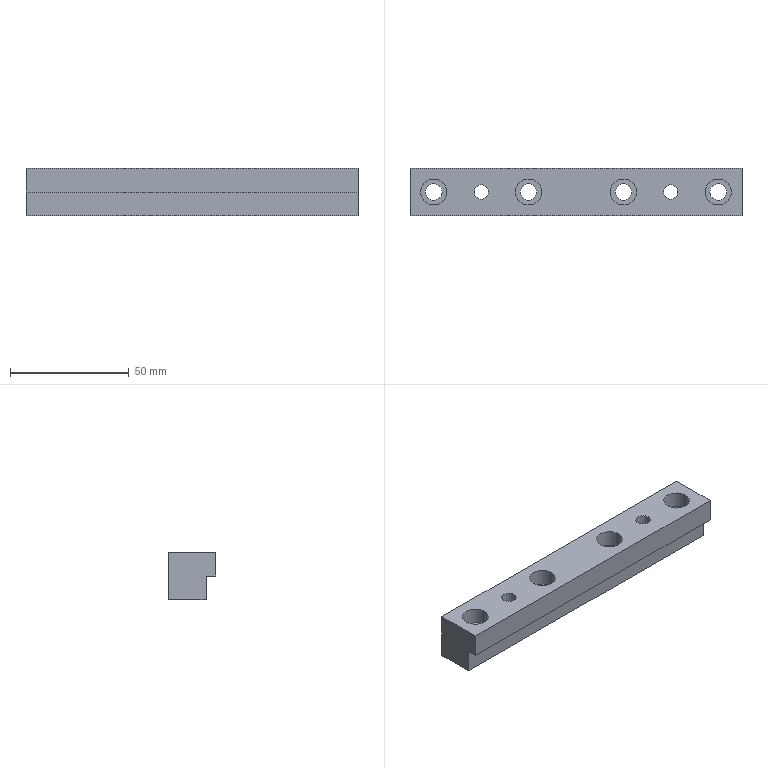Part | STEP file | 200 mesh_id1922 | 1 solid | 22 faces | box 140 x 20 x 20 mm | volume 44533 mm3 | plane 12 | cylinder 10 | commonest cylinder face diameters 7 x4 11 x4 6.01 x2
STEP:
#1=CARTESIAN_POINT('',(-16699.686,-3880.269,22.));
#2=VERTEX_POINT('',#1);
#3=CARTESIAN_POINT('',(-16839.686,-3880.269,22.));
#4=VERTEX_POINT('',#3);
#5=CARTESIAN_POINT('',(-16903.186,-3880.269,22.));
#6=DIRECTION('',(-1.,0.,0.));
#7=VECTOR('',#6,1.);
#8=LINE('',#5,#7);
#9=EDGE_CURVE('',#2,#4,#8,.T.);
#10=ORIENTED_EDGE('',*,*,#9,.F.);
#11=CARTESIAN_POINT('',(-16699.686,-3880.269,32.));
#12=VERTEX_POINT('',#11);
#13=CARTESIAN_POINT('',(-16699.686,-3880.269,12.));
#14=DIRECTION('',(0.,0.,-1.));
#15=VECTOR('',#14,1.);
#16=LINE('',#13,#15);
#17=EDGE_CURVE('',#12,#2,#16,.T.);
#18=ORIENTED_EDGE('',*,*,#17,.F.);
#19=CARTESIAN_POINT('',(-16839.686,-3880.269,32.));
#20=VERTEX_POINT('',#19);
#21=CARTESIAN_POINT('',(-16841.186,-3880.269,32.));
#22=DIRECTION('',(-1.,0.,0.));
#23=VECTOR('',#22,1.);
#24=LINE('',#21,#23);
#25=EDGE_CURVE('',#12,#20,#24,.T.);
#26=ORIENTED_EDGE('',*,*,#25,.T.);
#27=CARTESIAN_POINT('',(-16839.686,-3880.269,12.));
#28=DIRECTION('',(0.,0.,-1.));
#29=VECTOR('',#28,1.);
#30=LINE('',#27,#29);
#31=EDGE_CURVE('',#20,#4,#30,.T.);
#32=ORIENTED_EDGE('',*,*,#31,.T.);
#33=EDGE_LOOP('',(#10,#18,#26,#32));
#34=FACE_OUTER_BOUND('',#33,.T.);
#35=CARTESIAN_POINT('',(-16841.186,-3880.269,12.));
#36=DIRECTION('',(0.,1.,0.));
#37=DIRECTION('',(0.,0.,-1.));
#38=AXIS2_PLACEMENT_3D('',#35,#36,#37);
#39=PLANE('',#38);
#40=ADVANCED_FACE('',(#34),#39,.F.);
#41=CARTESIAN_POINT('',(-16699.686,-3876.219,12.));
#42=VERTEX_POINT('',#41);
#43=CARTESIAN_POINT('',(-16699.686,-3876.219,22.));
#44=VERTEX_POINT('',#43);
#45=CARTESIAN_POINT('',(-16699.686,-3876.219,22.));
#46=DIRECTION('',(0.,0.,1.));
#47=VECTOR('',#46,1.);
#48=LINE('',#45,#47);
#49=EDGE_CURVE('',#42,#44,#48,.T.);
#50=ORIENTED_EDGE('',*,*,#49,.F.);
#51=CARTESIAN_POINT('',(-16699.686,-3860.269,12.));
#52=VERTEX_POINT('',#51);
#53=CARTESIAN_POINT('',(-16699.686,-3870.269,12.));
#54=DIRECTION('',(0.,-1.,0.));
#55=VECTOR('',#54,1.);
#56=LINE('',#53,#55);
#57=EDGE_CURVE('',#52,#42,#56,.T.);
#58=ORIENTED_EDGE('',*,*,#57,.F.);
#59=CARTESIAN_POINT('',(-16699.686,-3860.269,32.));
#60=VERTEX_POINT('',#59);
#61=CARTESIAN_POINT('',(-16699.686,-3860.269,12.));
#62=DIRECTION('',(0.,0.,-1.));
#63=VECTOR('',#62,1.);
#64=LINE('',#61,#63);
#65=EDGE_CURVE('',#60,#52,#64,.T.);
#66=ORIENTED_EDGE('',*,*,#65,.F.);
#67=CARTESIAN_POINT('',(-16699.686,-3870.269,32.));
#68=DIRECTION('',(0.,-1.,0.));
#69=VECTOR('',#68,1.);
#70=LINE('',#67,#69);
#71=EDGE_CURVE('',#60,#12,#70,.T.);
#72=ORIENTED_EDGE('',*,*,#71,.T.);
#73=ORIENTED_EDGE('',*,*,#17,.T.);
#74=CARTESIAN_POINT('',(-16699.686,-3880.269,22.));
#75=DIRECTION('',(0.,-1.,0.));
#76=VECTOR('',#75,1.);
#77=LINE('',#74,#76);
#78=EDGE_CURVE('',#44,#2,#77,.T.);
#79=ORIENTED_EDGE('',*,*,#78,.F.);
#80=EDGE_LOOP('',(#50,#58,#66,#72,#73,#79));
#81=FACE_OUTER_BOUND('',#80,.T.);
#82=CARTESIAN_POINT('',(-16699.686,-3880.269,12.));
#83=DIRECTION('',(-1.,0.,0.));
#84=DIRECTION('',(0.,1.,0.));
#85=AXIS2_PLACEMENT_3D('',#82,#83,#84);
#86=PLANE('',#85);
#87=ADVANCED_FACE('',(#81),#86,.F.);
#88=CARTESIAN_POINT('',(-16826.186,-3870.269,12.));
#89=VERTEX_POINT('',#88);
#90=CARTESIAN_POINT('',(-16829.686,-3870.269,12.));
#91=DIRECTION('',(0.,0.,1.));
#92=DIRECTION('',(1.,0.,0.));
#93=AXIS2_PLACEMENT_3D('',#90,#91,#92);
#94=CIRCLE('',#93,3.5);
#95=EDGE_CURVE('',#89,#89,#94,.T.);
#96=ORIENTED_EDGE('',*,*,#95,.T.);
#97=EDGE_LOOP('',(#96));
#98=FACE_BOUND('',#97,.T.);
#99=CARTESIAN_POINT('',(-16806.681,-3870.269,12.));
#100=VERTEX_POINT('',#99);
#101=CARTESIAN_POINT('',(-16809.686,-3870.269,12.));
#102=DIRECTION('',(0.,0.,1.));
#103=DIRECTION('',(1.,0.,0.));
#104=AXIS2_PLACEMENT_3D('',#101,#102,#103);
#105=CIRCLE('',#104,3.005);
#106=EDGE_CURVE('',#100,#100,#105,.T.);
#107=ORIENTED_EDGE('',*,*,#106,.T.);
#108=EDGE_LOOP('',(#107));
#109=FACE_BOUND('',#108,.T.);
#110=CARTESIAN_POINT('',(-16786.186,-3870.269,12.));
#111=VERTEX_POINT('',#110);
#112=CARTESIAN_POINT('',(-16789.686,-3870.269,12.));
#113=DIRECTION('',(0.,0.,1.));
#114=DIRECTION('',(1.,0.,0.));
#115=AXIS2_PLACEMENT_3D('',#112,#113,#114);
#116=CIRCLE('',#115,3.5);
#117=EDGE_CURVE('',#111,#111,#116,.T.);
#118=ORIENTED_EDGE('',*,*,#117,.T.);
#119=EDGE_LOOP('',(#118));
#120=FACE_BOUND('',#119,.T.);
#121=CARTESIAN_POINT('',(-16726.681,-3870.269,12.));
#122=VERTEX_POINT('',#121);
#123=CARTESIAN_POINT('',(-16729.686,-3870.269,12.));
#124=DIRECTION('',(0.,0.,1.));
#125=DIRECTION('',(1.,0.,0.));
#126=AXIS2_PLACEMENT_3D('',#123,#124,#125);
#127=CIRCLE('',#126,3.005);
#128=EDGE_CURVE('',#122,#122,#127,.T.);
#129=ORIENTED_EDGE('',*,*,#128,.T.);
#130=EDGE_LOOP('',(#129));
#131=FACE_BOUND('',#130,.T.);
#132=CARTESIAN_POINT('',(-16746.186,-3870.269,12.));
#133=VERTEX_POINT('',#132);
#134=CARTESIAN_POINT('',(-16749.686,-3870.269,12.));
#135=DIRECTION('',(0.,0.,1.));
#136=DIRECTION('',(1.,0.,0.));
#137=AXIS2_PLACEMENT_3D('',#134,#135,#136);
#138=CIRCLE('',#137,3.5);
#139=EDGE_CURVE('',#133,#133,#138,.T.);
#140=ORIENTED_EDGE('',*,*,#139,.T.);
#141=EDGE_LOOP('',(#140));
#142=FACE_BOUND('',#141,.T.);
#143=CARTESIAN_POINT('',(-16706.186,-3870.269,12.));
#144=VERTEX_POINT('',#143);
#145=CARTESIAN_POINT('',(-16709.686,-3870.269,12.));
#146=DIRECTION('',(0.,0.,1.));
#147=DIRECTION('',(1.,0.,0.));
#148=AXIS2_PLACEMENT_3D('',#145,#146,#147);
#149=CIRCLE('',#148,3.5);
#150=EDGE_CURVE('',#144,#144,#149,.T.);
#151=ORIENTED_EDGE('',*,*,#150,.T.);
#152=EDGE_LOOP('',(#151));
#153=FACE_BOUND('',#152,.T.);
#154=CARTESIAN_POINT('',(-16839.686,-3876.219,12.));
#155=VERTEX_POINT('',#154);
#156=CARTESIAN_POINT('',(-16903.186,-3876.219,12.));
#157=DIRECTION('',(1.,0.,0.));
#158=VECTOR('',#157,1.);
#159=LINE('',#156,#158);
#160=EDGE_CURVE('',#155,#42,#159,.T.);
#161=ORIENTED_EDGE('',*,*,#160,.F.);
#162=CARTESIAN_POINT('',(-16839.686,-3860.269,12.));
#163=VERTEX_POINT('',#162);
#164=CARTESIAN_POINT('',(-16839.686,-3870.269,12.));
#165=DIRECTION('',(0.,1.,0.));
#166=VECTOR('',#165,1.);
#167=LINE('',#164,#166);
#168=EDGE_CURVE('',#155,#163,#167,.T.);
#169=ORIENTED_EDGE('',*,*,#168,.T.);
#170=CARTESIAN_POINT('',(-16703.186,-3860.269,12.));
#171=DIRECTION('',(1.,0.,0.));
#172=VECTOR('',#171,1.);
#173=LINE('',#170,#172);
#174=EDGE_CURVE('',#163,#52,#173,.T.);
#175=ORIENTED_EDGE('',*,*,#174,.T.);
#176=ORIENTED_EDGE('',*,*,#57,.T.);
#177=EDGE_LOOP('',(#161,#169,#175,#176));
#178=FACE_BOUND('',#177,.T.);
#179=CARTESIAN_POINT('',(-16709.686,-3870.269,12.));
#180=DIRECTION('',(0.,0.,1.));
#181=DIRECTION('',(1.,0.,0.));
#182=AXIS2_PLACEMENT_3D('',#179,#180,#181);
#183=PLANE('',#182);
#184=ADVANCED_FACE('',(#98,#109,#120,#131,#142,#153,#178),#183,.F.);
#185=CARTESIAN_POINT('',(-16839.686,-3876.219,22.));
#186=VERTEX_POINT('',#185);
#187=CARTESIAN_POINT('',(-16839.686,-3860.269,22.));
#188=DIRECTION('',(0.,-1.,0.));
#189=VECTOR('',#188,1.);
#190=LINE('',#187,#189);
#191=EDGE_CURVE('',#186,#4,#190,.T.);
#192=ORIENTED_EDGE('',*,*,#191,.T.);
#193=ORIENTED_EDGE('',*,*,#31,.F.);
#194=CARTESIAN_POINT('',(-16839.686,-3860.269,32.));
#195=VERTEX_POINT('',#194);
#196=CARTESIAN_POINT('',(-16839.686,-3870.269,32.));
#197=DIRECTION('',(0.,1.,0.));
#198=VECTOR('',#197,1.);
#199=LINE('',#196,#198);
#200=EDGE_CURVE('',#20,#195,#199,.T.);
#201=ORIENTED_EDGE('',*,*,#200,.T.);
#202=CARTESIAN_POINT('',(-16839.686,-3860.269,12.));
#203=DIRECTION('',(0.,0.,-1.));
#204=VECTOR('',#203,1.);
#205=LINE('',#202,#204);
#206=EDGE_CURVE('',#195,#163,#205,.T.);
#207=ORIENTED_EDGE('',*,*,#206,.T.);
#208=ORIENTED_EDGE('',*,*,#168,.F.);
#209=CARTESIAN_POINT('',(-16839.686,-3876.219,12.));
#210=DIRECTION('',(0.,0.,1.));
#211=VECTOR('',#210,1.);
#212=LINE('',#209,#211);
#213=EDGE_CURVE('',#155,#186,#212,.T.);
#214=ORIENTED_EDGE('',*,*,#213,.T.);
#215=EDGE_LOOP('',(#192,#193,#201,#207,#208,#214));
#216=FACE_OUTER_BOUND('',#215,.T.);
#217=CARTESIAN_POINT('',(-16839.686,-3860.269,12.));
#218=DIRECTION('',(1.,0.,0.));
#219=DIRECTION('',(0.,0.,-1.));
#220=AXIS2_PLACEMENT_3D('',#217,#218,#219);
#221=PLANE('',#220);
#222=ADVANCED_FACE('',(#216),#221,.F.);
#223=ORIENTED_EDGE('',*,*,#106,.F.);
#224=EDGE_LOOP('',(#223));
#225=FACE_BOUND('',#224,.T.);
#226=CARTESIAN_POINT('',(-16806.681,-3870.269,32.));
#227=VERTEX_POINT('',#226);
#228=CARTESIAN_POINT('',(-16809.686,-3870.269,32.));
#229=DIRECTION('',(0.,0.,1.));
#230=DIRECTION('',(1.,0.,0.));
#231=AXIS2_PLACEMENT_3D('',#228,#229,#230);
#232=CIRCLE('',#231,3.005);
#233=EDGE_CURVE('',#227,#227,#232,.T.);
#234=ORIENTED_EDGE('',*,*,#233,.T.);
#235=EDGE_LOOP('',(#234));
#236=FACE_BOUND('',#235,.T.);
#237=CARTESIAN_POINT('',(-16809.686,-3870.269,12.));
#238=DIRECTION('',(0.,0.,1.));
#239=DIRECTION('',(1.,0.,0.));
#240=AXIS2_PLACEMENT_3D('',#237,#238,#239);
#241=CYLINDRICAL_SURFACE('',#240,3.005);
#242=ADVANCED_FACE('',(#225,#236),#241,.F.);
#243=CARTESIAN_POINT('',(-16793.186,-3870.269,25.));
#244=VERTEX_POINT('',#243);
#245=CARTESIAN_POINT('',(-16789.686,-3870.269,25.));
#246=DIRECTION('',(0.,0.,1.));
#247=DIRECTION('',(-1.,0.,0.));
#248=AXIS2_PLACEMENT_3D('',#245,#246,#247);
#249=CIRCLE('',#248,3.5);
#250=EDGE_CURVE('',#244,#244,#249,.T.);
#251=ORIENTED_EDGE('',*,*,#250,.T.);
#252=EDGE_LOOP('',(#251));
#253=FACE_BOUND('',#252,.T.);
#254=ORIENTED_EDGE('',*,*,#117,.F.);
#255=EDGE_LOOP('',(#254));
#256=FACE_BOUND('',#255,.T.);
#257=CARTESIAN_POINT('',(-16789.686,-3870.269,12.));
#258=DIRECTION('',(0.,0.,1.));
#259=DIRECTION('',(1.,0.,0.));
#260=AXIS2_PLACEMENT_3D('',#257,#258,#259);
#261=CYLINDRICAL_SURFACE('',#260,3.5);
#262=ADVANCED_FACE('',(#253,#256),#261,.F.);
#263=ORIENTED_EDGE('',*,*,#128,.F.);
#264=EDGE_LOOP('',(#263));
#265=FACE_BOUND('',#264,.T.);
#266=CARTESIAN_POINT('',(-16726.681,-3870.269,32.));
#267=VERTEX_POINT('',#266);
#268=CARTESIAN_POINT('',(-16729.686,-3870.269,32.));
#269=DIRECTION('',(0.,0.,1.));
#270=DIRECTION('',(1.,0.,0.));
#271=AXIS2_PLACEMENT_3D('',#268,#269,#270);
#272=CIRCLE('',#271,3.005);
#273=EDGE_CURVE('',#267,#267,#272,.T.);
#274=ORIENTED_EDGE('',*,*,#273,.T.);
#275=EDGE_LOOP('',(#274));
#276=FACE_BOUND('',#275,.T.);
#277=CARTESIAN_POINT('',(-16729.686,-3870.269,12.));
#278=DIRECTION('',(0.,0.,1.));
#279=DIRECTION('',(1.,0.,0.));
#280=AXIS2_PLACEMENT_3D('',#277,#278,#279);
#281=CYLINDRICAL_SURFACE('',#280,3.005);
#282=ADVANCED_FACE('',(#265,#276),#281,.F.);
#283=CARTESIAN_POINT('',(-16753.186,-3870.269,25.));
#284=VERTEX_POINT('',#283);
#285=CARTESIAN_POINT('',(-16749.686,-3870.269,25.));
#286=DIRECTION('',(0.,0.,1.));
#287=DIRECTION('',(-1.,0.,0.));
#288=AXIS2_PLACEMENT_3D('',#285,#286,#287);
#289=CIRCLE('',#288,3.5);
#290=EDGE_CURVE('',#284,#284,#289,.T.);
#291=ORIENTED_EDGE('',*,*,#290,.T.);
#292=EDGE_LOOP('',(#291));
#293=FACE_BOUND('',#292,.T.);
#294=ORIENTED_EDGE('',*,*,#139,.F.);
#295=EDGE_LOOP('',(#294));
#296=FACE_BOUND('',#295,.T.);
#297=CARTESIAN_POINT('',(-16749.686,-3870.269,12.));
#298=DIRECTION('',(0.,0.,1.));
#299=DIRECTION('',(1.,0.,0.));
#300=AXIS2_PLACEMENT_3D('',#297,#298,#299);
#301=CYLINDRICAL_SURFACE('',#300,3.5);
#302=ADVANCED_FACE('',(#293,#296),#301,.F.);
#303=CARTESIAN_POINT('',(-16713.186,-3870.269,25.));
#304=VERTEX_POINT('',#303);
#305=CARTESIAN_POINT('',(-16709.686,-3870.269,25.));
#306=DIRECTION('',(0.,0.,1.));
#307=DIRECTION('',(-1.,0.,0.));
#308=AXIS2_PLACEMENT_3D('',#305,#306,#307);
#309=CIRCLE('',#308,3.5);
#310=EDGE_CURVE('',#304,#304,#309,.T.);
#311=ORIENTED_EDGE('',*,*,#310,.T.);
#312=EDGE_LOOP('',(#311));
#313=FACE_BOUND('',#312,.T.);
#314=ORIENTED_EDGE('',*,*,#150,.F.);
#315=EDGE_LOOP('',(#314));
#316=FACE_BOUND('',#315,.T.);
#317=CARTESIAN_POINT('',(-16709.686,-3870.269,12.));
#318=DIRECTION('',(0.,0.,1.));
#319=DIRECTION('',(1.,0.,0.));
#320=AXIS2_PLACEMENT_3D('',#317,#318,#319);
#321=CYLINDRICAL_SURFACE('',#320,3.5);
#322=ADVANCED_FACE('',(#313,#316),#321,.F.);
#323=CARTESIAN_POINT('',(-16703.186,-3860.269,32.));
#324=DIRECTION('',(1.,0.,0.));
#325=VECTOR('',#324,1.);
#326=LINE('',#323,#325);
#327=EDGE_CURVE('',#195,#60,#326,.T.);
#328=ORIENTED_EDGE('',*,*,#327,.T.);
#329=ORIENTED_EDGE('',*,*,#65,.T.);
#330=ORIENTED_EDGE('',*,*,#174,.F.);
#331=ORIENTED_EDGE('',*,*,#206,.F.);
#332=EDGE_LOOP('',(#328,#329,#330,#331));
#333=FACE_OUTER_BOUND('',#332,.T.);
#334=CARTESIAN_POINT('',(-16703.186,-3860.269,12.));
#335=DIRECTION('',(0.,-1.,0.));
#336=DIRECTION('',(-1.,0.,0.));
#337=AXIS2_PLACEMENT_3D('',#334,#335,#336);
#338=PLANE('',#337);
#339=ADVANCED_FACE('',(#333),#338,.F.);
#340=CARTESIAN_POINT('',(-16833.186,-3870.269,25.));
#341=VERTEX_POINT('',#340);
#342=CARTESIAN_POINT('',(-16829.686,-3870.269,25.));
#343=DIRECTION('',(0.,0.,1.));
#344=DIRECTION('',(-1.,0.,0.));
#345=AXIS2_PLACEMENT_3D('',#342,#343,#344);
#346=CIRCLE('',#345,3.5);
#347=EDGE_CURVE('',#341,#341,#346,.T.);
#348=ORIENTED_EDGE('',*,*,#347,.T.);
#349=EDGE_LOOP('',(#348));
#350=FACE_BOUND('',#349,.T.);
#351=ORIENTED_EDGE('',*,*,#95,.F.);
#352=EDGE_LOOP('',(#351));
#353=FACE_BOUND('',#352,.T.);
#354=CARTESIAN_POINT('',(-16829.686,-3870.269,12.));
#355=DIRECTION('',(0.,0.,1.));
#356=DIRECTION('',(1.,0.,0.));
#357=AXIS2_PLACEMENT_3D('',#354,#355,#356);
#358=CYLINDRICAL_SURFACE('',#357,3.5);
#359=ADVANCED_FACE('',(#350,#353),#358,.F.);
#360=CARTESIAN_POINT('',(-16704.186,-3870.269,32.));
#361=VERTEX_POINT('',#360);
#362=CARTESIAN_POINT('',(-16709.686,-3870.269,32.));
#363=DIRECTION('',(0.,0.,-1.));
#364=DIRECTION('',(1.,0.,0.));
#365=AXIS2_PLACEMENT_3D('',#362,#363,#364);
#366=CIRCLE('',#365,5.5);
#367=EDGE_CURVE('',#361,#361,#366,.T.);
#368=ORIENTED_EDGE('',*,*,#367,.T.);
#369=EDGE_LOOP('',(#368));
#370=FACE_BOUND('',#369,.T.);
#371=CARTESIAN_POINT('',(-16744.186,-3870.269,32.));
#372=VERTEX_POINT('',#371);
#373=CARTESIAN_POINT('',(-16749.686,-3870.269,32.));
#374=DIRECTION('',(0.,0.,-1.));
#375=DIRECTION('',(1.,0.,0.));
#376=AXIS2_PLACEMENT_3D('',#373,#374,#375);
#377=CIRCLE('',#376,5.5);
#378=EDGE_CURVE('',#372,#372,#377,.T.);
#379=ORIENTED_EDGE('',*,*,#378,.T.);
#380=EDGE_LOOP('',(#379));
#381=FACE_BOUND('',#380,.T.);
#382=CARTESIAN_POINT('',(-16784.186,-3870.269,32.));
#383=VERTEX_POINT('',#382);
#384=CARTESIAN_POINT('',(-16789.686,-3870.269,32.));
#385=DIRECTION('',(0.,0.,-1.));
#386=DIRECTION('',(1.,0.,0.));
#387=AXIS2_PLACEMENT_3D('',#384,#385,#386);
#388=CIRCLE('',#387,5.5);
#389=EDGE_CURVE('',#383,#383,#388,.T.);
#390=ORIENTED_EDGE('',*,*,#389,.T.);
#391=EDGE_LOOP('',(#390));
#392=FACE_BOUND('',#391,.T.);
#393=CARTESIAN_POINT('',(-16824.186,-3870.269,32.));
#394=VERTEX_POINT('',#393);
#395=CARTESIAN_POINT('',(-16829.686,-3870.269,32.));
#396=DIRECTION('',(0.,0.,-1.));
#397=DIRECTION('',(1.,0.,0.));
#398=AXIS2_PLACEMENT_3D('',#395,#396,#397);
#399=CIRCLE('',#398,5.5);
#400=EDGE_CURVE('',#394,#394,#399,.T.);
#401=ORIENTED_EDGE('',*,*,#400,.T.);
#402=EDGE_LOOP('',(#401));
#403=FACE_BOUND('',#402,.T.);
#404=ORIENTED_EDGE('',*,*,#200,.F.);
#405=ORIENTED_EDGE('',*,*,#25,.F.);
#406=ORIENTED_EDGE('',*,*,#71,.F.);
#407=ORIENTED_EDGE('',*,*,#327,.F.);
#408=EDGE_LOOP('',(#404,#405,#406,#407));
#409=FACE_BOUND('',#408,.T.);
#410=ORIENTED_EDGE('',*,*,#273,.F.);
#411=EDGE_LOOP('',(#410));
#412=FACE_BOUND('',#411,.T.);
#413=ORIENTED_EDGE('',*,*,#233,.F.);
#414=EDGE_LOOP('',(#413));
#415=FACE_BOUND('',#414,.T.);
#416=CARTESIAN_POINT('',(-16709.686,-3870.269,32.));
#417=DIRECTION('',(0.,0.,1.));
#418=DIRECTION('',(1.,0.,0.));
#419=AXIS2_PLACEMENT_3D('',#416,#417,#418);
#420=PLANE('',#419);
#421=ADVANCED_FACE('',(#370,#381,#392,#403,#409,#412,#415),#420,.T.);
#422=ORIENTED_EDGE('',*,*,#213,.F.);
#423=ORIENTED_EDGE('',*,*,#160,.T.);
#424=ORIENTED_EDGE('',*,*,#49,.T.);
#425=CARTESIAN_POINT('',(-16903.186,-3876.219,22.));
#426=DIRECTION('',(-1.,0.,0.));
#427=VECTOR('',#426,1.);
#428=LINE('',#425,#427);
#429=EDGE_CURVE('',#44,#186,#428,.T.);
#430=ORIENTED_EDGE('',*,*,#429,.T.);
#431=EDGE_LOOP('',(#422,#423,#424,#430));
#432=FACE_OUTER_BOUND('',#431,.T.);
#433=CARTESIAN_POINT('',(-16903.186,-3876.219,22.));
#434=DIRECTION('',(0.,1.,0.));
#435=DIRECTION('',(1.,0.,0.));
#436=AXIS2_PLACEMENT_3D('',#433,#434,#435);
#437=PLANE('',#436);
#438=ADVANCED_FACE('',(#432),#437,.F.);
#439=ORIENTED_EDGE('',*,*,#191,.F.);
#440=ORIENTED_EDGE('',*,*,#429,.F.);
#441=ORIENTED_EDGE('',*,*,#78,.T.);
#442=ORIENTED_EDGE('',*,*,#9,.T.);
#443=EDGE_LOOP('',(#439,#440,#441,#442));
#444=FACE_OUTER_BOUND('',#443,.T.);
#445=CARTESIAN_POINT('',(-16903.186,-3880.269,22.));
#446=DIRECTION('',(0.,0.,1.));
#447=DIRECTION('',(0.,-1.,0.));
#448=AXIS2_PLACEMENT_3D('',#445,#446,#447);
#449=PLANE('',#448);
#450=ADVANCED_FACE('',(#444),#449,.F.);
#451=CARTESIAN_POINT('',(-16835.186,-3870.269,25.));
#452=VERTEX_POINT('',#451);
#453=CARTESIAN_POINT('',(-16829.686,-3870.269,25.));
#454=DIRECTION('',(0.,0.,-1.));
#455=DIRECTION('',(-1.,0.,0.));
#456=AXIS2_PLACEMENT_3D('',#453,#454,#455);
#457=CIRCLE('',#456,5.5);
#458=EDGE_CURVE('',#452,#452,#457,.T.);
#459=ORIENTED_EDGE('',*,*,#458,.F.);
#460=EDGE_LOOP('',(#459));
#461=FACE_BOUND('',#460,.T.);
#462=ORIENTED_EDGE('',*,*,#347,.F.);
#463=EDGE_LOOP('',(#462));
#464=FACE_BOUND('',#463,.T.);
#465=CARTESIAN_POINT('',(-16829.686,-3870.269,25.));
#466=DIRECTION('',(0.,0.,-1.));
#467=DIRECTION('',(-1.,0.,0.));
#468=AXIS2_PLACEMENT_3D('',#465,#466,#467);
#469=PLANE('',#468);
#470=ADVANCED_FACE('',(#461,#464),#469,.F.);
#471=ORIENTED_EDGE('',*,*,#458,.T.);
#472=EDGE_LOOP('',(#471));
#473=FACE_BOUND('',#472,.T.);
#474=ORIENTED_EDGE('',*,*,#400,.F.);
#475=EDGE_LOOP('',(#474));
#476=FACE_BOUND('',#475,.T.);
#477=CARTESIAN_POINT('',(-16829.686,-3870.269,32.));
#478=DIRECTION('',(0.,0.,-1.));
#479=DIRECTION('',(1.,0.,0.));
#480=AXIS2_PLACEMENT_3D('',#477,#478,#479);
#481=CYLINDRICAL_SURFACE('',#480,5.5);
#482=ADVANCED_FACE('',(#473,#476),#481,.F.);
#483=CARTESIAN_POINT('',(-16795.186,-3870.269,25.));
#484=VERTEX_POINT('',#483);
#485=CARTESIAN_POINT('',(-16789.686,-3870.269,25.));
#486=DIRECTION('',(0.,0.,-1.));
#487=DIRECTION('',(-1.,0.,0.));
#488=AXIS2_PLACEMENT_3D('',#485,#486,#487);
#489=CIRCLE('',#488,5.5);
#490=EDGE_CURVE('',#484,#484,#489,.T.);
#491=ORIENTED_EDGE('',*,*,#490,.F.);
#492=EDGE_LOOP('',(#491));
#493=FACE_BOUND('',#492,.T.);
#494=ORIENTED_EDGE('',*,*,#250,.F.);
#495=EDGE_LOOP('',(#494));
#496=FACE_BOUND('',#495,.T.);
#497=CARTESIAN_POINT('',(-16789.686,-3870.269,25.));
#498=DIRECTION('',(0.,0.,-1.));
#499=DIRECTION('',(-1.,0.,0.));
#500=AXIS2_PLACEMENT_3D('',#497,#498,#499);
#501=PLANE('',#500);
#502=ADVANCED_FACE('',(#493,#496),#501,.F.);
#503=ORIENTED_EDGE('',*,*,#490,.T.);
#504=EDGE_LOOP('',(#503));
#505=FACE_BOUND('',#504,.T.);
#506=ORIENTED_EDGE('',*,*,#389,.F.);
#507=EDGE_LOOP('',(#506));
#508=FACE_BOUND('',#507,.T.);
#509=CARTESIAN_POINT('',(-16789.686,-3870.269,32.));
#510=DIRECTION('',(0.,0.,-1.));
#511=DIRECTION('',(1.,0.,0.));
#512=AXIS2_PLACEMENT_3D('',#509,#510,#511);
#513=CYLINDRICAL_SURFACE('',#512,5.5);
#514=ADVANCED_FACE('',(#505,#508),#513,.F.);
#515=CARTESIAN_POINT('',(-16755.186,-3870.269,25.));
#516=VERTEX_POINT('',#515);
#517=CARTESIAN_POINT('',(-16749.686,-3870.269,25.));
#518=DIRECTION('',(0.,0.,-1.));
#519=DIRECTION('',(-1.,0.,0.));
#520=AXIS2_PLACEMENT_3D('',#517,#518,#519);
#521=CIRCLE('',#520,5.5);
#522=EDGE_CURVE('',#516,#516,#521,.T.);
#523=ORIENTED_EDGE('',*,*,#522,.F.);
#524=EDGE_LOOP('',(#523));
#525=FACE_BOUND('',#524,.T.);
#526=ORIENTED_EDGE('',*,*,#290,.F.);
#527=EDGE_LOOP('',(#526));
#528=FACE_BOUND('',#527,.T.);
#529=CARTESIAN_POINT('',(-16749.686,-3870.269,25.));
#530=DIRECTION('',(0.,0.,-1.));
#531=DIRECTION('',(-1.,0.,0.));
#532=AXIS2_PLACEMENT_3D('',#529,#530,#531);
#533=PLANE('',#532);
#534=ADVANCED_FACE('',(#525,#528),#533,.F.);
#535=ORIENTED_EDGE('',*,*,#522,.T.);
#536=EDGE_LOOP('',(#535));
#537=FACE_BOUND('',#536,.T.);
#538=ORIENTED_EDGE('',*,*,#378,.F.);
#539=EDGE_LOOP('',(#538));
#540=FACE_BOUND('',#539,.T.);
#541=CARTESIAN_POINT('',(-16749.686,-3870.269,32.));
#542=DIRECTION('',(0.,0.,-1.));
#543=DIRECTION('',(1.,0.,0.));
#544=AXIS2_PLACEMENT_3D('',#541,#542,#543);
#545=CYLINDRICAL_SURFACE('',#544,5.5);
#546=ADVANCED_FACE('',(#537,#540),#545,.F.);
#547=CARTESIAN_POINT('',(-16715.186,-3870.269,25.));
#548=VERTEX_POINT('',#547);
#549=CARTESIAN_POINT('',(-16709.686,-3870.269,25.));
#550=DIRECTION('',(0.,0.,-1.));
#551=DIRECTION('',(-1.,0.,0.));
#552=AXIS2_PLACEMENT_3D('',#549,#550,#551);
#553=CIRCLE('',#552,5.5);
#554=EDGE_CURVE('',#548,#548,#553,.T.);
#555=ORIENTED_EDGE('',*,*,#554,.F.);
#556=EDGE_LOOP('',(#555));
#557=FACE_BOUND('',#556,.T.);
#558=ORIENTED_EDGE('',*,*,#310,.F.);
#559=EDGE_LOOP('',(#558));
#560=FACE_BOUND('',#559,.T.);
#561=CARTESIAN_POINT('',(-16709.686,-3870.269,25.));
#562=DIRECTION('',(0.,0.,-1.));
#563=DIRECTION('',(-1.,0.,0.));
#564=AXIS2_PLACEMENT_3D('',#561,#562,#563);
#565=PLANE('',#564);
#566=ADVANCED_FACE('',(#557,#560),#565,.F.);
#567=ORIENTED_EDGE('',*,*,#554,.T.);
#568=EDGE_LOOP('',(#567));
#569=FACE_BOUND('',#568,.T.);
#570=ORIENTED_EDGE('',*,*,#367,.F.);
#571=EDGE_LOOP('',(#570));
#572=FACE_BOUND('',#571,.T.);
#573=CARTESIAN_POINT('',(-16709.686,-3870.269,32.));
#574=DIRECTION('',(0.,0.,-1.));
#575=DIRECTION('',(1.,0.,0.));
#576=AXIS2_PLACEMENT_3D('',#573,#574,#575);
#577=CYLINDRICAL_SURFACE('',#576,5.5);
#578=ADVANCED_FACE('',(#569,#572),#577,.F.);
#579=CLOSED_SHELL('',(#40,#87,#184,#222,#242,#262,#282,#302,#322,#339,#359,#421,#438,#450,#470,#482,#502,#514,#534,#546,#566,#578));
#580=MANIFOLD_SOLID_BREP('',#579);
#581=(LENGTH_UNIT()NAMED_UNIT(*)SI_UNIT(.MILLI.,.METRE.));
#582=UNCERTAINTY_MEASURE_WITH_UNIT(LENGTH_MEASURE(0.00002),#581,'','');
#583=(NAMED_UNIT(*)PLANE_ANGLE_UNIT()SI_UNIT($,.RADIAN.));
#584=PLANE_ANGLE_MEASURE_WITH_UNIT(PLANE_ANGLE_MEASURE(0.01745),#583);
#585=DIMENSIONAL_EXPONENTS(0.,0.,0.,0.,0.,0.,0.);
#586=(CONVERSION_BASED_UNIT('DEGREE',#584)NAMED_UNIT(#585)PLANE_ANGLE_UNIT());
#587=(NAMED_UNIT(*)SI_UNIT($,.STERADIAN.)SOLID_ANGLE_UNIT());
#588=(GEOMETRIC_REPRESENTATION_CONTEXT(3)GLOBAL_UNCERTAINTY_ASSIGNED_CONTEXT((#582))GLOBAL_UNIT_ASSIGNED_CONTEXT((#581,#586,#587))REPRESENTATION_CONTEXT('',''));
#589=ADVANCED_BREP_SHAPE_REPRESENTATION('',(#580),#588);